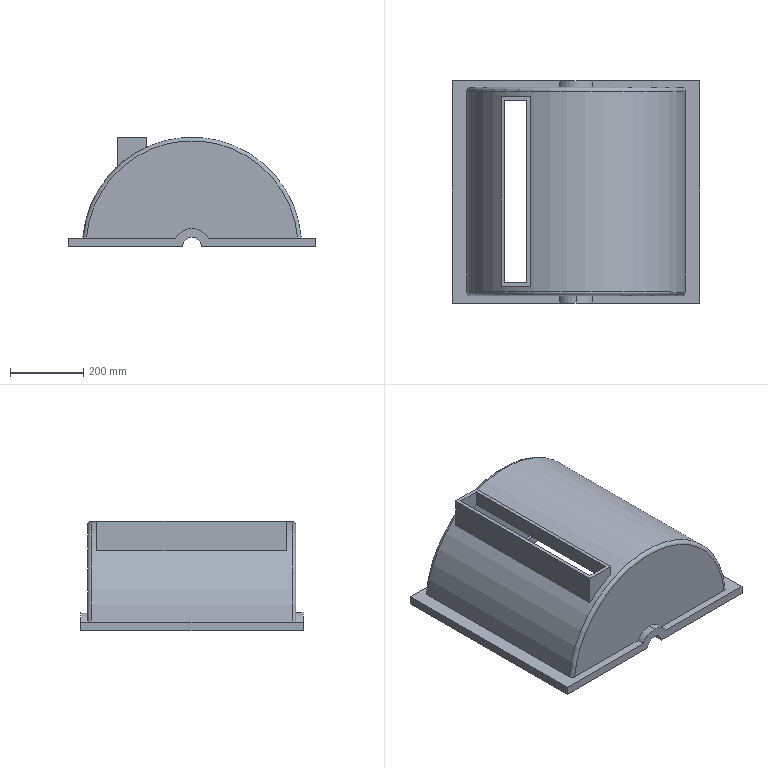Part | SolidWorks | features ICE 11, MirrorPattern 4, Extrusion 1, Fillet 1 | 1 solid | 41 faces | box 677.491 x 608 x 300 mm | volume 10187902 mm3 | plane 25 | cylinder 14 | torus 2 | commonest cylinder face diameters 100 x6 52 x4 556 x2 580 x1 600 x1
STEP:
#1=CARTESIAN_POINT('',(5.246,268.,26.));
#2=VERTEX_POINT('',#1);
#3=CARTESIAN_POINT('',(31.246,268.,0.));
#4=VERTEX_POINT('',#3);
#5=CARTESIAN_POINT('',(5.246,268.,0.));
#6=DIRECTION('',(0.,1.,0.));
#7=DIRECTION('',(0.,0.,1.));
#8=AXIS2_PLACEMENT_3D('',#5,#6,#7);
#9=CIRCLE('',#8,26.);
#10=EDGE_CURVE('',#2,#4,#9,.T.);
#11=ORIENTED_EDGE('',*,*,#10,.F.);
#12=CARTESIAN_POINT('',(5.246,304.,26.));
#13=VERTEX_POINT('',#12);
#14=CARTESIAN_POINT('',(5.246,-304.,26.));
#15=DIRECTION('',(0.,1.,0.));
#16=VECTOR('',#15,1000.);
#17=LINE('',#14,#16);
#18=EDGE_CURVE('',#2,#13,#17,.T.);
#19=ORIENTED_EDGE('',*,*,#18,.T.);
#20=CARTESIAN_POINT('',(31.246,304.,0.));
#21=VERTEX_POINT('',#20);
#22=CARTESIAN_POINT('',(5.246,304.,0.));
#23=DIRECTION('',(0.,1.,0.));
#24=DIRECTION('',(0.,0.,1.));
#25=AXIS2_PLACEMENT_3D('',#22,#23,#24);
#26=CIRCLE('',#25,26.);
#27=EDGE_CURVE('',#13,#21,#26,.T.);
#28=ORIENTED_EDGE('',*,*,#27,.T.);
#29=CARTESIAN_POINT('',(31.246,-304.,0.));
#30=DIRECTION('',(0.,1.,0.));
#31=VECTOR('',#30,1000.);
#32=LINE('',#29,#31);
#33=EDGE_CURVE('',#4,#21,#32,.T.);
#34=ORIENTED_EDGE('',*,*,#33,.F.);
#35=EDGE_LOOP('',(#11,#19,#28,#34));
#36=FACE_OUTER_BOUND('',#35,.T.);
#37=CARTESIAN_POINT('',(5.246,-304.,0.));
#38=DIRECTION('',(0.,1.,0.));
#39=DIRECTION('',(0.,0.,1.));
#40=AXIS2_PLACEMENT_3D('',#37,#38,#39);
#41=CYLINDRICAL_SURFACE('',#40,26.);
#42=ADVANCED_FACE('',(#36),#41,.F.);
#43=CARTESIAN_POINT('',(31.246,-304.,0.));
#44=VERTEX_POINT('',#43);
#45=CARTESIAN_POINT('',(5.246,-304.,26.));
#46=VERTEX_POINT('',#45);
#47=CARTESIAN_POINT('',(5.246,-304.,0.));
#48=DIRECTION('',(0.,-1.,0.));
#49=DIRECTION('',(0.,0.,-1.));
#50=AXIS2_PLACEMENT_3D('',#47,#48,#49);
#51=CIRCLE('',#50,26.);
#52=EDGE_CURVE('',#44,#46,#51,.T.);
#53=ORIENTED_EDGE('',*,*,#52,.T.);
#54=CARTESIAN_POINT('',(5.246,-268.,26.));
#55=VERTEX_POINT('',#54);
#56=CARTESIAN_POINT('',(5.246,-304.,26.));
#57=DIRECTION('',(0.,1.,0.));
#58=VECTOR('',#57,1000.);
#59=LINE('',#56,#58);
#60=EDGE_CURVE('',#46,#55,#59,.T.);
#61=ORIENTED_EDGE('',*,*,#60,.T.);
#62=CARTESIAN_POINT('',(31.246,-268.,0.));
#63=VERTEX_POINT('',#62);
#64=CARTESIAN_POINT('',(5.246,-268.,0.));
#65=DIRECTION('',(0.,-1.,0.));
#66=DIRECTION('',(0.,0.,-1.));
#67=AXIS2_PLACEMENT_3D('',#64,#65,#66);
#68=CIRCLE('',#67,26.);
#69=EDGE_CURVE('',#63,#55,#68,.T.);
#70=ORIENTED_EDGE('',*,*,#69,.F.);
#71=CARTESIAN_POINT('',(31.246,-304.,0.));
#72=DIRECTION('',(0.,1.,0.));
#73=VECTOR('',#72,1000.);
#74=LINE('',#71,#73);
#75=EDGE_CURVE('',#44,#63,#74,.T.);
#76=ORIENTED_EDGE('',*,*,#75,.F.);
#77=EDGE_LOOP('',(#53,#61,#70,#76));
#78=FACE_OUTER_BOUND('',#77,.T.);
#79=CARTESIAN_POINT('',(5.246,-304.,0.));
#80=DIRECTION('',(0.,1.,0.));
#81=DIRECTION('',(0.,0.,1.));
#82=AXIS2_PLACEMENT_3D('',#79,#80,#81);
#83=CYLINDRICAL_SURFACE('',#82,26.);
#84=ADVANCED_FACE('',(#78),#83,.F.);
#85=CARTESIAN_POINT('',(-38.618,-304.,24.));
#86=VERTEX_POINT('',#85);
#87=CARTESIAN_POINT('',(5.246,-304.,50.));
#88=VERTEX_POINT('',#87);
#89=CARTESIAN_POINT('',(5.246,-304.,0.));
#90=DIRECTION('',(0.,1.,0.));
#91=DIRECTION('',(0.,0.,1.));
#92=AXIS2_PLACEMENT_3D('',#89,#90,#91);
#93=CIRCLE('',#92,50.);
#94=EDGE_CURVE('',#86,#88,#93,.T.);
#95=ORIENTED_EDGE('',*,*,#94,.T.);
#96=CARTESIAN_POINT('',(5.246,-284.,50.));
#97=VERTEX_POINT('',#96);
#98=CARTESIAN_POINT('',(5.246,-304.,50.));
#99=DIRECTION('',(0.,1.,0.));
#100=VECTOR('',#99,1000.);
#101=LINE('',#98,#100);
#102=EDGE_CURVE('',#88,#97,#101,.T.);
#103=ORIENTED_EDGE('',*,*,#102,.T.);
#104=CARTESIAN_POINT('',(-38.618,-284.,24.));
#105=VERTEX_POINT('',#104);
#106=CARTESIAN_POINT('',(5.246,-284.,0.));
#107=DIRECTION('',(0.,1.,0.));
#108=DIRECTION('',(0.,0.,-1.));
#109=AXIS2_PLACEMENT_3D('',#106,#107,#108);
#110=CIRCLE('',#109,50.);
#111=EDGE_CURVE('',#105,#97,#110,.T.);
#112=ORIENTED_EDGE('',*,*,#111,.F.);
#113=CARTESIAN_POINT('',(-38.618,-304.,24.));
#114=DIRECTION('',(0.,1.,0.));
#115=VECTOR('',#114,1000.);
#116=LINE('',#113,#115);
#117=EDGE_CURVE('',#86,#105,#116,.T.);
#118=ORIENTED_EDGE('',*,*,#117,.F.);
#119=EDGE_LOOP('',(#95,#103,#112,#118));
#120=FACE_OUTER_BOUND('',#119,.T.);
#121=CARTESIAN_POINT('',(5.246,-304.,0.));
#122=DIRECTION('',(0.,1.,0.));
#123=DIRECTION('',(0.,0.,1.));
#124=AXIS2_PLACEMENT_3D('',#121,#122,#123);
#125=CYLINDRICAL_SURFACE('',#124,50.);
#126=ADVANCED_FACE('',(#120),#125,.T.);
#127=CARTESIAN_POINT('',(-38.618,-274.,24.));
#128=VERTEX_POINT('',#127);
#129=CARTESIAN_POINT('',(5.246,-274.,50.));
#130=VERTEX_POINT('',#129);
#131=CARTESIAN_POINT('',(5.246,-274.,0.));
#132=DIRECTION('',(0.,1.,0.));
#133=DIRECTION('',(0.,0.,-1.));
#134=AXIS2_PLACEMENT_3D('',#131,#132,#133);
#135=CIRCLE('',#134,50.);
#136=EDGE_CURVE('',#128,#130,#135,.T.);
#137=ORIENTED_EDGE('',*,*,#136,.T.);
#138=CARTESIAN_POINT('',(5.246,-268.,50.));
#139=VERTEX_POINT('',#138);
#140=CARTESIAN_POINT('',(5.246,-304.,50.));
#141=DIRECTION('',(0.,1.,0.));
#142=VECTOR('',#141,1000.);
#143=LINE('',#140,#142);
#144=EDGE_CURVE('',#130,#139,#143,.T.);
#145=ORIENTED_EDGE('',*,*,#144,.T.);
#146=CARTESIAN_POINT('',(-38.618,-268.,24.));
#147=VERTEX_POINT('',#146);
#148=CARTESIAN_POINT('',(5.246,-268.,0.));
#149=DIRECTION('',(0.,1.,0.));
#150=DIRECTION('',(0.,0.,-1.));
#151=AXIS2_PLACEMENT_3D('',#148,#149,#150);
#152=CIRCLE('',#151,50.);
#153=EDGE_CURVE('',#147,#139,#152,.T.);
#154=ORIENTED_EDGE('',*,*,#153,.F.);
#155=CARTESIAN_POINT('',(-38.618,-304.,24.));
#156=DIRECTION('',(0.,1.,0.));
#157=VECTOR('',#156,1000.);
#158=LINE('',#155,#157);
#159=EDGE_CURVE('',#128,#147,#158,.T.);
#160=ORIENTED_EDGE('',*,*,#159,.F.);
#161=EDGE_LOOP('',(#137,#145,#154,#160));
#162=FACE_OUTER_BOUND('',#161,.T.);
#163=CARTESIAN_POINT('',(5.246,-304.,0.));
#164=DIRECTION('',(0.,1.,0.));
#165=DIRECTION('',(0.,0.,1.));
#166=AXIS2_PLACEMENT_3D('',#163,#164,#165);
#167=CYLINDRICAL_SURFACE('',#166,50.);
#168=ADVANCED_FACE('',(#162),#167,.T.);
#169=CARTESIAN_POINT('',(-38.618,276.,24.));
#170=VERTEX_POINT('',#169);
#171=CARTESIAN_POINT('',(-283.759,276.,24.));
#172=VERTEX_POINT('',#171);
#173=CARTESIAN_POINT('',(-293.793,276.,24.));
#174=DIRECTION('',(-1.,0.,0.));
#175=VECTOR('',#174,1000.);
#176=LINE('',#173,#175);
#177=EDGE_CURVE('',#170,#172,#176,.T.);
#178=ORIENTED_EDGE('',*,*,#177,.T.);
#179=CARTESIAN_POINT('',(-283.759,-274.,24.));
#180=VERTEX_POINT('',#179);
#181=CARTESIAN_POINT('',(-283.759,286.,24.));
#182=DIRECTION('',(0.,-1.,0.));
#183=VECTOR('',#182,1000.);
#184=LINE('',#181,#183);
#185=EDGE_CURVE('',#172,#180,#184,.T.);
#186=ORIENTED_EDGE('',*,*,#185,.T.);
#187=CARTESIAN_POINT('',(-38.618,-274.,24.));
#188=DIRECTION('',(1.,0.,0.));
#189=VECTOR('',#188,1000.);
#190=LINE('',#187,#189);
#191=EDGE_CURVE('',#180,#128,#190,.T.);
#192=ORIENTED_EDGE('',*,*,#191,.T.);
#193=ORIENTED_EDGE('',*,*,#159,.T.);
#194=CARTESIAN_POINT('',(-276.962,-268.,24.));
#195=VERTEX_POINT('',#194);
#196=CARTESIAN_POINT('',(0.,-268.,24.));
#197=DIRECTION('',(1.,0.,0.));
#198=VECTOR('',#197,1000.);
#199=LINE('',#196,#198);
#200=EDGE_CURVE('',#195,#147,#199,.T.);
#201=ORIENTED_EDGE('',*,*,#200,.F.);
#202=CARTESIAN_POINT('',(-276.962,268.,24.));
#203=VERTEX_POINT('',#202);
#204=CARTESIAN_POINT('',(-276.962,278.,24.));
#205=DIRECTION('',(0.,1.,0.));
#206=VECTOR('',#205,1000.);
#207=LINE('',#204,#206);
#208=EDGE_CURVE('',#195,#203,#207,.T.);
#209=ORIENTED_EDGE('',*,*,#208,.T.);
#210=CARTESIAN_POINT('',(-38.618,268.,24.));
#211=VERTEX_POINT('',#210);
#212=CARTESIAN_POINT('',(0.,268.,24.));
#213=DIRECTION('',(-1.,0.,0.));
#214=VECTOR('',#213,1000.);
#215=LINE('',#212,#214);
#216=EDGE_CURVE('',#211,#203,#215,.T.);
#217=ORIENTED_EDGE('',*,*,#216,.F.);
#218=CARTESIAN_POINT('',(-38.618,304.,24.));
#219=DIRECTION('',(0.,-1.,0.));
#220=VECTOR('',#219,1000.);
#221=LINE('',#218,#220);
#222=EDGE_CURVE('',#170,#211,#221,.T.);
#223=ORIENTED_EDGE('',*,*,#222,.F.);
#224=EDGE_LOOP('',(#178,#186,#192,#193,#201,#209,#217,#223));
#225=FACE_OUTER_BOUND('',#224,.T.);
#226=CARTESIAN_POINT('',(0.,278.,24.));
#227=DIRECTION('',(0.,0.,-1.));
#228=DIRECTION('',(-1.,0.,0.));
#229=AXIS2_PLACEMENT_3D('',#226,#227,#228);
#230=PLANE('',#229);
#231=ADVANCED_FACE('',(#225),#230,.F.);
#232=CARTESIAN_POINT('',(294.251,276.,24.));
#233=VERTEX_POINT('',#232);
#234=CARTESIAN_POINT('',(294.251,-274.,24.));
#235=VERTEX_POINT('',#234);
#236=CARTESIAN_POINT('',(294.251,286.,24.));
#237=DIRECTION('',(0.,-1.,0.));
#238=VECTOR('',#237,1000.);
#239=LINE('',#236,#238);
#240=EDGE_CURVE('',#233,#235,#239,.T.);
#241=ORIENTED_EDGE('',*,*,#240,.F.);
#242=CARTESIAN_POINT('',(49.109,276.,24.));
#243=VERTEX_POINT('',#242);
#244=CARTESIAN_POINT('',(304.284,276.,24.));
#245=DIRECTION('',(-1.,0.,0.));
#246=VECTOR('',#245,1000.);
#247=LINE('',#244,#246);
#248=EDGE_CURVE('',#233,#243,#247,.T.);
#249=ORIENTED_EDGE('',*,*,#248,.T.);
#250=CARTESIAN_POINT('',(49.109,268.,24.));
#251=VERTEX_POINT('',#250);
#252=CARTESIAN_POINT('',(49.109,304.,24.));
#253=DIRECTION('',(0.,-1.,0.));
#254=VECTOR('',#253,1000.);
#255=LINE('',#252,#254);
#256=EDGE_CURVE('',#243,#251,#255,.T.);
#257=ORIENTED_EDGE('',*,*,#256,.T.);
#258=CARTESIAN_POINT('',(287.453,268.,24.));
#259=VERTEX_POINT('',#258);
#260=CARTESIAN_POINT('',(0.,268.,24.));
#261=DIRECTION('',(-1.,0.,0.));
#262=VECTOR('',#261,1000.);
#263=LINE('',#260,#262);
#264=EDGE_CURVE('',#259,#251,#263,.T.);
#265=ORIENTED_EDGE('',*,*,#264,.F.);
#266=CARTESIAN_POINT('',(287.453,-268.,24.));
#267=VERTEX_POINT('',#266);
#268=CARTESIAN_POINT('',(287.453,278.,24.));
#269=DIRECTION('',(0.,1.,0.));
#270=VECTOR('',#269,1000.);
#271=LINE('',#268,#270);
#272=EDGE_CURVE('',#267,#259,#271,.T.);
#273=ORIENTED_EDGE('',*,*,#272,.F.);
#274=CARTESIAN_POINT('',(49.109,-268.,24.));
#275=VERTEX_POINT('',#274);
#276=CARTESIAN_POINT('',(0.,-268.,24.));
#277=DIRECTION('',(1.,0.,0.));
#278=VECTOR('',#277,1000.);
#279=LINE('',#276,#278);
#280=EDGE_CURVE('',#275,#267,#279,.T.);
#281=ORIENTED_EDGE('',*,*,#280,.F.);
#282=CARTESIAN_POINT('',(49.109,-274.,24.));
#283=VERTEX_POINT('',#282);
#284=CARTESIAN_POINT('',(49.109,-304.,24.));
#285=DIRECTION('',(0.,1.,0.));
#286=VECTOR('',#285,1000.);
#287=LINE('',#284,#286);
#288=EDGE_CURVE('',#283,#275,#287,.T.);
#289=ORIENTED_EDGE('',*,*,#288,.F.);
#290=CARTESIAN_POINT('',(49.109,-274.,24.));
#291=DIRECTION('',(1.,0.,0.));
#292=VECTOR('',#291,1000.);
#293=LINE('',#290,#292);
#294=EDGE_CURVE('',#283,#235,#293,.T.);
#295=ORIENTED_EDGE('',*,*,#294,.T.);
#296=EDGE_LOOP('',(#241,#249,#257,#265,#273,#281,#289,#295));
#297=FACE_OUTER_BOUND('',#296,.T.);
#298=CARTESIAN_POINT('',(10.491,278.,24.));
#299=DIRECTION('',(0.,0.,1.));
#300=DIRECTION('',(1.,0.,0.));
#301=AXIS2_PLACEMENT_3D('',#298,#299,#300);
#302=PLANE('',#301);
#303=ADVANCED_FACE('',(#297),#302,.T.);
#304=CARTESIAN_POINT('',(-190.,-249.,214.427));
#305=VERTEX_POINT('',#304);
#306=CARTESIAN_POINT('',(-190.,251.,214.427));
#307=VERTEX_POINT('',#306);
#308=CARTESIAN_POINT('',(-190.,286.,214.427));
#309=DIRECTION('',(0.,1.,0.));
#310=VECTOR('',#309,1000.);
#311=LINE('',#308,#310);
#312=EDGE_CURVE('',#305,#307,#311,.T.);
#313=ORIENTED_EDGE('',*,*,#312,.F.);
#314=CARTESIAN_POINT('',(-129.462,-249.,256.815));
#315=VERTEX_POINT('',#314);
#316=CARTESIAN_POINT('',(5.246,-249.,0.));
#317=DIRECTION('',(0.,-1.,0.));
#318=DIRECTION('',(0.,0.,-1.));
#319=AXIS2_PLACEMENT_3D('',#316,#317,#318);
#320=CIRCLE('',#319,290.);
#321=EDGE_CURVE('',#315,#305,#320,.T.);
#322=ORIENTED_EDGE('',*,*,#321,.F.);
#323=CARTESIAN_POINT('',(-129.462,251.,256.815));
#324=VERTEX_POINT('',#323);
#325=CARTESIAN_POINT('',(-129.462,286.,256.815));
#326=DIRECTION('',(0.,-1.,0.));
#327=VECTOR('',#326,1000.);
#328=LINE('',#325,#327);
#329=EDGE_CURVE('',#324,#315,#328,.T.);
#330=ORIENTED_EDGE('',*,*,#329,.F.);
#331=CARTESIAN_POINT('',(5.246,251.,0.));
#332=DIRECTION('',(0.,1.,0.));
#333=DIRECTION('',(0.,0.,1.));
#334=AXIS2_PLACEMENT_3D('',#331,#332,#333);
#335=CIRCLE('',#334,290.);
#336=EDGE_CURVE('',#307,#324,#335,.T.);
#337=ORIENTED_EDGE('',*,*,#336,.F.);
#338=EDGE_LOOP('',(#313,#322,#330,#337));
#339=FACE_BOUND('',#338,.T.);
#340=ORIENTED_EDGE('',*,*,#185,.F.);
#341=CARTESIAN_POINT('',(5.246,276.,0.));
#342=DIRECTION('',(0.,1.,0.));
#343=DIRECTION('',(0.,0.,1.));
#344=AXIS2_PLACEMENT_3D('',#341,#342,#343);
#345=CIRCLE('',#344,290.);
#346=EDGE_CURVE('',#172,#233,#345,.T.);
#347=ORIENTED_EDGE('',*,*,#346,.T.);
#348=ORIENTED_EDGE('',*,*,#240,.T.);
#349=CARTESIAN_POINT('',(5.246,-274.,0.));
#350=DIRECTION('',(0.,-1.,0.));
#351=DIRECTION('',(0.,0.,-1.));
#352=AXIS2_PLACEMENT_3D('',#349,#350,#351);
#353=CIRCLE('',#352,290.);
#354=EDGE_CURVE('',#235,#180,#353,.T.);
#355=ORIENTED_EDGE('',*,*,#354,.T.);
#356=EDGE_LOOP('',(#340,#347,#348,#355));
#357=FACE_OUTER_BOUND('',#356,.T.);
#358=CARTESIAN_POINT('',(5.246,286.,0.));
#359=DIRECTION('',(0.,-1.,0.));
#360=DIRECTION('',(0.,0.,-1.));
#361=AXIS2_PLACEMENT_3D('',#358,#359,#360);
#362=CYLINDRICAL_SURFACE('',#361,290.);
#363=ADVANCED_FACE('',(#339,#357),#362,.F.);
#364=CARTESIAN_POINT('',(5.246,276.,0.));
#365=DIRECTION('',(0.,-1.,0.));
#366=DIRECTION('',(0.,0.,1.));
#367=AXIS2_PLACEMENT_3D('',#364,#365,#366);
#368=CIRCLE('',#367,50.);
#369=EDGE_CURVE('',#243,#170,#368,.T.);
#370=ORIENTED_EDGE('',*,*,#369,.T.);
#371=ORIENTED_EDGE('',*,*,#222,.T.);
#372=CARTESIAN_POINT('',(5.246,268.,0.));
#373=DIRECTION('',(0.,-1.,0.));
#374=DIRECTION('',(0.,0.,1.));
#375=AXIS2_PLACEMENT_3D('',#372,#373,#374);
#376=CIRCLE('',#375,50.);
#377=EDGE_CURVE('',#251,#211,#376,.T.);
#378=ORIENTED_EDGE('',*,*,#377,.F.);
#379=ORIENTED_EDGE('',*,*,#256,.F.);
#380=EDGE_LOOP('',(#370,#371,#378,#379));
#381=FACE_OUTER_BOUND('',#380,.T.);
#382=CARTESIAN_POINT('',(5.246,304.,0.));
#383=DIRECTION('',(0.,-1.,0.));
#384=DIRECTION('',(0.,0.,-1.));
#385=AXIS2_PLACEMENT_3D('',#382,#383,#384);
#386=CYLINDRICAL_SURFACE('',#385,50.);
#387=ADVANCED_FACE('',(#381),#386,.T.);
#388=CARTESIAN_POINT('',(-38.618,286.,24.));
#389=VERTEX_POINT('',#388);
#390=CARTESIAN_POINT('',(-283.759,286.,24.));
#391=VERTEX_POINT('',#390);
#392=CARTESIAN_POINT('',(0.,286.,24.));
#393=DIRECTION('',(-1.,0.,0.));
#394=VECTOR('',#393,1000.);
#395=LINE('',#392,#394);
#396=EDGE_CURVE('',#389,#391,#395,.T.);
#397=ORIENTED_EDGE('',*,*,#396,.F.);
#398=CARTESIAN_POINT('',(-38.618,304.,24.));
#399=VERTEX_POINT('',#398);
#400=CARTESIAN_POINT('',(-38.618,304.,24.));
#401=DIRECTION('',(0.,-1.,0.));
#402=VECTOR('',#401,1000.);
#403=LINE('',#400,#402);
#404=EDGE_CURVE('',#399,#389,#403,.T.);
#405=ORIENTED_EDGE('',*,*,#404,.F.);
#406=CARTESIAN_POINT('',(-333.5,304.,24.));
#407=VERTEX_POINT('',#406);
#408=CARTESIAN_POINT('',(-333.5,304.,24.));
#409=DIRECTION('',(1.,0.,0.));
#410=VECTOR('',#409,1000.);
#411=LINE('',#408,#410);
#412=EDGE_CURVE('',#407,#399,#411,.T.);
#413=ORIENTED_EDGE('',*,*,#412,.F.);
#414=CARTESIAN_POINT('',(-333.5,-304.,24.));
#415=VERTEX_POINT('',#414);
#416=CARTESIAN_POINT('',(-333.5,278.,24.));
#417=DIRECTION('',(0.,-1.,0.));
#418=VECTOR('',#417,1000.);
#419=LINE('',#416,#418);
#420=EDGE_CURVE('',#407,#415,#419,.T.);
#421=ORIENTED_EDGE('',*,*,#420,.T.);
#422=CARTESIAN_POINT('',(-333.5,-304.,24.));
#423=DIRECTION('',(1.,0.,0.));
#424=VECTOR('',#423,1000.);
#425=LINE('',#422,#424);
#426=EDGE_CURVE('',#415,#86,#425,.T.);
#427=ORIENTED_EDGE('',*,*,#426,.T.);
#428=ORIENTED_EDGE('',*,*,#117,.T.);
#429=CARTESIAN_POINT('',(-283.759,-284.,24.));
#430=VERTEX_POINT('',#429);
#431=CARTESIAN_POINT('',(0.,-284.,24.));
#432=DIRECTION('',(-1.,0.,0.));
#433=VECTOR('',#432,1000.);
#434=LINE('',#431,#433);
#435=EDGE_CURVE('',#105,#430,#434,.T.);
#436=ORIENTED_EDGE('',*,*,#435,.T.);
#437=CARTESIAN_POINT('',(-293.793,-274.,24.));
#438=VERTEX_POINT('',#437);
#439=CARTESIAN_POINT('',(-283.759,-284.,24.));
#440=CARTESIAN_POINT('',(-284.421,-284.,24.));
#441=CARTESIAN_POINT('',(-285.071,-283.935,24.));
#442=CARTESIAN_POINT('',(-286.031,-283.746,24.));
#443=CARTESIAN_POINT('',(-286.348,-283.667,24.));
#444=CARTESIAN_POINT('',(-286.977,-283.477,24.));
#445=CARTESIAN_POINT('',(-287.29,-283.366,24.));
#446=CARTESIAN_POINT('',(-288.2,-282.991,24.));
#447=CARTESIAN_POINT('',(-288.776,-282.685,24.));
#448=CARTESIAN_POINT('',(-289.866,-281.962,24.));
#449=CARTESIAN_POINT('',(-290.383,-281.54,24.));
#450=CARTESIAN_POINT('',(-291.309,-280.619,24.));
#451=CARTESIAN_POINT('',(-291.725,-280.116,24.));
#452=CARTESIAN_POINT('',(-292.276,-279.298,24.));
#453=CARTESIAN_POINT('',(-292.447,-279.014,24.));
#454=CARTESIAN_POINT('',(-292.758,-278.436,24.));
#455=CARTESIAN_POINT('',(-293.038,-277.847,24.));
#456=CARTESIAN_POINT('',(-293.26,-277.233,24.));
#457=CARTESIAN_POINT('',(-293.451,-276.607,24.));
#458=CARTESIAN_POINT('',(-293.533,-276.286,24.));
#459=CARTESIAN_POINT('',(-293.728,-275.316,24.));
#460=CARTESIAN_POINT('',(-293.793,-274.661,24.));
#461=CARTESIAN_POINT('',(-293.793,-274.,24.));
#462=B_SPLINE_CURVE_WITH_KNOTS('',3,(#439,#440,#441,#442,#443,#444,#445,#446,#447,#448,#449,#450,#451,#452,#453,#454,#455,#456,#457,#458,#459,#460,#461),.UNSPECIFIED.,.F.,.F.,(4,2,2,2,2,2,2,2,1,2,2,4),(0.,0.001956,0.002934,0.003912,0.005868,0.007824,0.00978,0.01076,0.01174,0.01271,0.01369,0.01565),.UNSPECIFIED.);
#463=EDGE_CURVE('',#430,#438,#462,.T.);
#464=ORIENTED_EDGE('',*,*,#463,.T.);
#465=CARTESIAN_POINT('',(-293.793,276.,24.));
#466=VERTEX_POINT('',#465);
#467=CARTESIAN_POINT('',(-293.793,286.,24.));
#468=DIRECTION('',(0.,1.,0.));
#469=VECTOR('',#468,1000.);
#470=LINE('',#467,#469);
#471=EDGE_CURVE('',#438,#466,#470,.T.);
#472=ORIENTED_EDGE('',*,*,#471,.T.);
#473=CARTESIAN_POINT('',(-293.793,276.,24.));
#474=CARTESIAN_POINT('',(-293.793,276.661,24.));
#475=CARTESIAN_POINT('',(-293.728,277.312,24.));
#476=CARTESIAN_POINT('',(-293.536,278.271,24.));
#477=CARTESIAN_POINT('',(-293.457,278.588,24.));
#478=CARTESIAN_POINT('',(-293.265,279.217,24.));
#479=CARTESIAN_POINT('',(-293.153,279.529,24.));
#480=CARTESIAN_POINT('',(-292.775,280.438,24.));
#481=CARTESIAN_POINT('',(-292.466,281.012,24.));
#482=CARTESIAN_POINT('',(-291.92,281.828,24.));
#483=CARTESIAN_POINT('',(-291.723,282.093,24.));
#484=CARTESIAN_POINT('',(-291.303,282.602,24.));
#485=CARTESIAN_POINT('',(-291.082,282.844,24.));
#486=CARTESIAN_POINT('',(-290.388,283.535,24.));
#487=CARTESIAN_POINT('',(-289.883,283.949,24.));
#488=CARTESIAN_POINT('',(-289.061,284.496,24.));
#489=CARTESIAN_POINT('',(-288.777,284.666,24.));
#490=CARTESIAN_POINT('',(-288.198,284.974,24.));
#491=CARTESIAN_POINT('',(-287.608,285.252,24.));
#492=CARTESIAN_POINT('',(-286.993,285.472,24.));
#493=CARTESIAN_POINT('',(-286.366,285.662,24.));
#494=CARTESIAN_POINT('',(-286.045,285.743,24.));
#495=CARTESIAN_POINT('',(-285.075,285.935,24.));
#496=CARTESIAN_POINT('',(-284.421,286.,24.));
#497=CARTESIAN_POINT('',(-283.759,286.,24.));
#498=B_SPLINE_CURVE_WITH_KNOTS('',3,(#473,#474,#475,#476,#477,#478,#479,#480,#481,#482,#483,#484,#485,#486,#487,#488,#489,#490,#491,#492,#493,#494,#495,#496,#497),.UNSPECIFIED.,.F.,.F.,(4,2,2,2,2,2,2,2,2,1,2,2,4),(0.,0.001956,0.002934,0.003912,0.005868,0.006846,0.007824,0.00978,0.01076,0.01174,0.01271,0.01369,0.01565),.UNSPECIFIED.);
#499=EDGE_CURVE('',#466,#391,#498,.T.);
#500=ORIENTED_EDGE('',*,*,#499,.T.);
#501=EDGE_LOOP('',(#397,#405,#413,#421,#427,#428,#436,#464,#472,#500));
#502=FACE_OUTER_BOUND('',#501,.T.);
#503=CARTESIAN_POINT('',(0.,278.,24.));
#504=DIRECTION('',(0.,0.,-1.));
#505=DIRECTION('',(-1.,0.,0.));
#506=AXIS2_PLACEMENT_3D('',#503,#504,#505);
#507=PLANE('',#506);
#508=ADVANCED_FACE('',(#502),#507,.F.);
#509=CARTESIAN_POINT('',(49.109,304.,24.));
#510=VERTEX_POINT('',#509);
#511=CARTESIAN_POINT('',(49.109,286.,24.));
#512=VERTEX_POINT('',#511);
#513=CARTESIAN_POINT('',(49.109,304.,24.));
#514=DIRECTION('',(0.,-1.,0.));
#515=VECTOR('',#514,1000.);
#516=LINE('',#513,#515);
#517=EDGE_CURVE('',#510,#512,#516,.T.);
#518=ORIENTED_EDGE('',*,*,#517,.T.);
#519=CARTESIAN_POINT('',(294.251,286.,24.));
#520=VERTEX_POINT('',#519);
#521=CARTESIAN_POINT('',(10.491,286.,24.));
#522=DIRECTION('',(1.,0.,0.));
#523=VECTOR('',#522,1000.);
#524=LINE('',#521,#523);
#525=EDGE_CURVE('',#512,#520,#524,.T.);
#526=ORIENTED_EDGE('',*,*,#525,.T.);
#527=CARTESIAN_POINT('',(304.284,276.,24.));
#528=VERTEX_POINT('',#527);
#529=CARTESIAN_POINT('',(294.251,286.,24.));
#530=CARTESIAN_POINT('',(294.912,286.,24.));
#531=CARTESIAN_POINT('',(295.563,285.935,24.));
#532=CARTESIAN_POINT('',(296.522,285.746,24.));
#533=CARTESIAN_POINT('',(296.84,285.667,24.));
#534=CARTESIAN_POINT('',(297.469,285.477,24.));
#535=CARTESIAN_POINT('',(297.782,285.366,24.));
#536=CARTESIAN_POINT('',(298.692,284.991,24.));
#537=CARTESIAN_POINT('',(299.268,284.685,24.));
#538=CARTESIAN_POINT('',(300.357,283.962,24.));
#539=CARTESIAN_POINT('',(300.874,283.54,24.));
#540=CARTESIAN_POINT('',(301.8,282.619,24.));
#541=CARTESIAN_POINT('',(302.216,282.116,24.));
#542=CARTESIAN_POINT('',(302.767,281.298,24.));
#543=CARTESIAN_POINT('',(302.938,281.014,24.));
#544=CARTESIAN_POINT('',(303.249,280.436,24.));
#545=CARTESIAN_POINT('',(303.53,279.847,24.));
#546=CARTESIAN_POINT('',(303.751,279.233,24.));
#547=CARTESIAN_POINT('',(303.943,278.607,24.));
#548=CARTESIAN_POINT('',(304.024,278.286,24.));
#549=CARTESIAN_POINT('',(304.219,277.316,24.));
#550=CARTESIAN_POINT('',(304.284,276.661,24.));
#551=CARTESIAN_POINT('',(304.284,276.,24.));
#552=B_SPLINE_CURVE_WITH_KNOTS('',3,(#529,#530,#531,#532,#533,#534,#535,#536,#537,#538,#539,#540,#541,#542,#543,#544,#545,#546,#547,#548,#549,#550,#551),.UNSPECIFIED.,.F.,.F.,(4,2,2,2,2,2,2,2,1,2,2,4),(0.,0.001956,0.002934,0.003912,0.005868,0.007824,0.00978,0.01076,0.01174,0.01271,0.01369,0.01565),.UNSPECIFIED.);
#553=EDGE_CURVE('',#520,#528,#552,.T.);
#554=ORIENTED_EDGE('',*,*,#553,.T.);
#555=CARTESIAN_POINT('',(304.284,-274.,24.));
#556=VERTEX_POINT('',#555);
#557=CARTESIAN_POINT('',(304.284,286.,24.));
#558=DIRECTION('',(0.,1.,0.));
#559=VECTOR('',#558,1000.);
#560=LINE('',#557,#559);
#561=EDGE_CURVE('',#556,#528,#560,.T.);
#562=ORIENTED_EDGE('',*,*,#561,.F.);
#563=CARTESIAN_POINT('',(294.251,-284.,24.));
#564=VERTEX_POINT('',#563);
#565=CARTESIAN_POINT('',(304.284,-274.,24.));
#566=CARTESIAN_POINT('',(304.284,-274.661,24.));
#567=CARTESIAN_POINT('',(304.219,-275.312,24.));
#568=CARTESIAN_POINT('',(304.027,-276.271,24.));
#569=CARTESIAN_POINT('',(303.948,-276.588,24.));
#570=CARTESIAN_POINT('',(303.757,-277.217,24.));
#571=CARTESIAN_POINT('',(303.644,-277.529,24.));
#572=CARTESIAN_POINT('',(303.266,-278.438,24.));
#573=CARTESIAN_POINT('',(302.958,-279.012,24.));
#574=CARTESIAN_POINT('',(302.411,-279.828,24.));
#575=CARTESIAN_POINT('',(302.214,-280.093,24.));
#576=CARTESIAN_POINT('',(301.794,-280.602,24.));
#577=CARTESIAN_POINT('',(301.574,-280.844,24.));
#578=CARTESIAN_POINT('',(300.88,-281.535,24.));
#579=CARTESIAN_POINT('',(300.375,-281.949,24.));
#580=CARTESIAN_POINT('',(299.553,-282.496,24.));
#581=CARTESIAN_POINT('',(299.268,-282.666,24.));
#582=CARTESIAN_POINT('',(298.69,-282.974,24.));
#583=CARTESIAN_POINT('',(298.099,-283.252,24.));
#584=CARTESIAN_POINT('',(297.485,-283.472,24.));
#585=CARTESIAN_POINT('',(296.858,-283.662,24.));
#586=CARTESIAN_POINT('',(296.537,-283.743,24.));
#587=CARTESIAN_POINT('',(295.566,-283.935,24.));
#588=CARTESIAN_POINT('',(294.912,-284.,24.));
#589=CARTESIAN_POINT('',(294.251,-284.,24.));
#590=B_SPLINE_CURVE_WITH_KNOTS('',3,(#565,#566,#567,#568,#569,#570,#571,#572,#573,#574,#575,#576,#577,#578,#579,#580,#581,#582,#583,#584,#585,#586,#587,#588,#589),.UNSPECIFIED.,.F.,.F.,(4,2,2,2,2,2,2,2,2,1,2,2,4),(0.,0.001956,0.002934,0.003912,0.005868,0.006846,0.007824,0.00978,0.01076,0.01174,0.01271,0.01369,0.01565),.UNSPECIFIED.);
#591=EDGE_CURVE('',#556,#564,#590,.T.);
#592=ORIENTED_EDGE('',*,*,#591,.T.);
#593=CARTESIAN_POINT('',(49.109,-284.,24.));
#594=VERTEX_POINT('',#593);
#595=CARTESIAN_POINT('',(10.491,-284.,24.));
#596=DIRECTION('',(1.,0.,0.));
#597=VECTOR('',#596,1000.);
#598=LINE('',#595,#597);
#599=EDGE_CURVE('',#594,#564,#598,.T.);
#600=ORIENTED_EDGE('',*,*,#599,.F.);
#601=CARTESIAN_POINT('',(49.109,-304.,24.));
#602=VERTEX_POINT('',#601);
#603=CARTESIAN_POINT('',(49.109,-304.,24.));
#604=DIRECTION('',(0.,1.,0.));
#605=VECTOR('',#604,1000.);
#606=LINE('',#603,#605);
#607=EDGE_CURVE('',#602,#594,#606,.T.);
#608=ORIENTED_EDGE('',*,*,#607,.F.);
#609=CARTESIAN_POINT('',(343.991,-304.,24.));
#610=VERTEX_POINT('',#609);
#611=CARTESIAN_POINT('',(343.991,-304.,24.));
#612=DIRECTION('',(-1.,0.,0.));
#613=VECTOR('',#612,1000.);
#614=LINE('',#611,#613);
#615=EDGE_CURVE('',#610,#602,#614,.T.);
#616=ORIENTED_EDGE('',*,*,#615,.F.);
#617=CARTESIAN_POINT('',(343.991,304.,24.));
#618=VERTEX_POINT('',#617);
#619=CARTESIAN_POINT('',(343.991,278.,24.));
#620=DIRECTION('',(0.,-1.,0.));
#621=VECTOR('',#620,1000.);
#622=LINE('',#619,#621);
#623=EDGE_CURVE('',#618,#610,#622,.T.);
#624=ORIENTED_EDGE('',*,*,#623,.F.);
#625=CARTESIAN_POINT('',(343.991,304.,24.));
#626=DIRECTION('',(1.,0.,0.));
#627=VECTOR('',#626,1000.);
#628=LINE('',#625,#627);
#629=EDGE_CURVE('',#510,#618,#628,.T.);
#630=ORIENTED_EDGE('',*,*,#629,.F.);
#631=EDGE_LOOP('',(#518,#526,#554,#562,#592,#600,#608,#616,#624,#630));
#632=FACE_OUTER_BOUND('',#631,.T.);
#633=CARTESIAN_POINT('',(10.491,278.,24.));
#634=DIRECTION('',(0.,0.,1.));
#635=DIRECTION('',(1.,0.,0.));
#636=AXIS2_PLACEMENT_3D('',#633,#634,#635);
#637=PLANE('',#636);
#638=ADVANCED_FACE('',(#632),#637,.T.);
#639=ORIENTED_EDGE('',*,*,#144,.F.);
#640=CARTESIAN_POINT('',(5.246,-274.,0.));
#641=DIRECTION('',(0.,1.,0.));
#642=DIRECTION('',(0.,0.,-1.));
#643=AXIS2_PLACEMENT_3D('',#640,#641,#642);
#644=CIRCLE('',#643,50.);
#645=EDGE_CURVE('',#130,#283,#644,.T.);
#646=ORIENTED_EDGE('',*,*,#645,.T.);
#647=ORIENTED_EDGE('',*,*,#288,.T.);
#648=CARTESIAN_POINT('',(5.246,-268.,0.));
#649=DIRECTION('',(0.,1.,0.));
#650=DIRECTION('',(0.,0.,-1.));
#651=AXIS2_PLACEMENT_3D('',#648,#649,#650);
#652=CIRCLE('',#651,50.);
#653=EDGE_CURVE('',#139,#275,#652,.T.);
#654=ORIENTED_EDGE('',*,*,#653,.F.);
#655=EDGE_LOOP('',(#639,#646,#647,#654));
#656=FACE_OUTER_BOUND('',#655,.T.);
#657=CARTESIAN_POINT('',(5.246,-304.,0.));
#658=DIRECTION('',(0.,1.,0.));
#659=DIRECTION('',(0.,0.,1.));
#660=AXIS2_PLACEMENT_3D('',#657,#658,#659);
#661=CYLINDRICAL_SURFACE('',#660,50.);
#662=ADVANCED_FACE('',(#656),#661,.T.);
#663=CARTESIAN_POINT('',(343.991,-304.,0.));
#664=VERTEX_POINT('',#663);
#665=CARTESIAN_POINT('',(-333.5,-304.,0.));
#666=DIRECTION('',(1.,0.,0.));
#667=VECTOR('',#666,1000.);
#668=LINE('',#665,#667);
#669=EDGE_CURVE('',#44,#664,#668,.T.);
#670=ORIENTED_EDGE('',*,*,#669,.F.);
#671=ORIENTED_EDGE('',*,*,#75,.T.);
#672=CARTESIAN_POINT('',(288.491,-268.,0.));
#673=VERTEX_POINT('',#672);
#674=CARTESIAN_POINT('',(-298.,-268.,0.));
#675=DIRECTION('',(-1.,0.,0.));
#676=VECTOR('',#675,1000.);
#677=LINE('',#674,#676);
#678=EDGE_CURVE('',#673,#63,#677,.T.);
#679=ORIENTED_EDGE('',*,*,#678,.F.);
#680=CARTESIAN_POINT('',(288.491,268.,0.));
#681=VERTEX_POINT('',#680);
#682=CARTESIAN_POINT('',(288.491,278.,0.));
#683=DIRECTION('',(0.,-1.,0.));
#684=VECTOR('',#683,1000.);
#685=LINE('',#682,#684);
#686=EDGE_CURVE('',#681,#673,#685,.T.);
#687=ORIENTED_EDGE('',*,*,#686,.F.);
#688=CARTESIAN_POINT('',(-298.,268.,0.));
#689=DIRECTION('',(-1.,0.,0.));
#690=VECTOR('',#689,1000.);
#691=LINE('',#688,#690);
#692=EDGE_CURVE('',#681,#4,#691,.T.);
#693=ORIENTED_EDGE('',*,*,#692,.T.);
#694=ORIENTED_EDGE('',*,*,#33,.T.);
#695=CARTESIAN_POINT('',(343.991,304.,0.));
#696=VERTEX_POINT('',#695);
#697=CARTESIAN_POINT('',(-333.5,304.,0.));
#698=DIRECTION('',(1.,0.,0.));
#699=VECTOR('',#698,1000.);
#700=LINE('',#697,#699);
#701=EDGE_CURVE('',#21,#696,#700,.T.);
#702=ORIENTED_EDGE('',*,*,#701,.T.);
#703=CARTESIAN_POINT('',(343.991,278.,0.));
#704=DIRECTION('',(0.,-1.,0.));
#705=VECTOR('',#704,1000.);
#706=LINE('',#703,#705);
#707=EDGE_CURVE('',#696,#664,#706,.T.);
#708=ORIENTED_EDGE('',*,*,#707,.T.);
#709=EDGE_LOOP('',(#670,#671,#679,#687,#693,#694,#702,#708));
#710=FACE_OUTER_BOUND('',#709,.T.);
#711=CARTESIAN_POINT('',(0.,278.,0.));
#712=DIRECTION('',(0.,0.,1.));
#713=DIRECTION('',(1.,0.,0.));
#714=AXIS2_PLACEMENT_3D('',#711,#712,#713);
#715=PLANE('',#714);
#716=ADVANCED_FACE('',(#710),#715,.F.);
#717=ORIENTED_EDGE('',*,*,#208,.F.);
#718=CARTESIAN_POINT('',(-278.,-268.,0.));
#719=VERTEX_POINT('',#718);
#720=CARTESIAN_POINT('',(0.,-268.,0.));
#721=DIRECTION('',(0.,-1.,0.));
#722=DIRECTION('',(0.,0.,-1.));
#723=AXIS2_PLACEMENT_3D('',#720,#721,#722);
#724=CIRCLE('',#723,278.);
#725=EDGE_CURVE('',#195,#719,#724,.T.);
#726=ORIENTED_EDGE('',*,*,#725,.T.);
#727=CARTESIAN_POINT('',(-278.,268.,0.));
#728=VERTEX_POINT('',#727);
#729=CARTESIAN_POINT('',(-278.,278.,0.));
#730=DIRECTION('',(0.,-1.,0.));
#731=VECTOR('',#730,1000.);
#732=LINE('',#729,#731);
#733=EDGE_CURVE('',#728,#719,#732,.T.);
#734=ORIENTED_EDGE('',*,*,#733,.F.);
#735=CARTESIAN_POINT('',(0.,268.,0.));
#736=DIRECTION('',(0.,1.,0.));
#737=DIRECTION('',(0.,0.,1.));
#738=AXIS2_PLACEMENT_3D('',#735,#736,#737);
#739=CIRCLE('',#738,278.);
#740=EDGE_CURVE('',#728,#203,#739,.T.);
#741=ORIENTED_EDGE('',*,*,#740,.T.);
#742=EDGE_LOOP('',(#717,#726,#734,#741));
#743=FACE_OUTER_BOUND('',#742,.T.);
#744=CARTESIAN_POINT('',(0.,278.,0.));
#745=DIRECTION('',(0.,-1.,0.));
#746=DIRECTION('',(0.,0.,-1.));
#747=AXIS2_PLACEMENT_3D('',#744,#745,#746);
#748=CYLINDRICAL_SURFACE('',#747,278.);
#749=ADVANCED_FACE('',(#743),#748,.F.);
#750=CARTESIAN_POINT('',(-333.5,304.,0.));
#751=VERTEX_POINT('',#750);
#752=CARTESIAN_POINT('',(-20.754,304.,0.));
#753=VERTEX_POINT('',#752);
#754=CARTESIAN_POINT('',(-333.5,304.,0.));
#755=DIRECTION('',(1.,0.,0.));
#756=VECTOR('',#755,1000.);
#757=LINE('',#754,#756);
#758=EDGE_CURVE('',#751,#753,#757,.T.);
#759=ORIENTED_EDGE('',*,*,#758,.T.);
#760=CARTESIAN_POINT('',(-20.754,268.,0.));
#761=VERTEX_POINT('',#760);
#762=CARTESIAN_POINT('',(-20.754,-304.,0.));
#763=DIRECTION('',(0.,-1.,0.));
#764=VECTOR('',#763,1000.);
#765=LINE('',#762,#764);
#766=EDGE_CURVE('',#753,#761,#765,.T.);
#767=ORIENTED_EDGE('',*,*,#766,.T.);
#768=CARTESIAN_POINT('',(-298.,268.,0.));
#769=DIRECTION('',(-1.,0.,0.));
#770=VECTOR('',#769,1000.);
#771=LINE('',#768,#770);
#772=EDGE_CURVE('',#761,#728,#771,.T.);
#773=ORIENTED_EDGE('',*,*,#772,.T.);
#774=ORIENTED_EDGE('',*,*,#733,.T.);
#775=CARTESIAN_POINT('',(-20.754,-268.,0.));
#776=VERTEX_POINT('',#775);
#777=CARTESIAN_POINT('',(-298.,-268.,0.));
#778=DIRECTION('',(-1.,0.,0.));
#779=VECTOR('',#778,1000.);
#780=LINE('',#777,#779);
#781=EDGE_CURVE('',#776,#719,#780,.T.);
#782=ORIENTED_EDGE('',*,*,#781,.F.);
#783=CARTESIAN_POINT('',(-20.754,-304.,0.));
#784=VERTEX_POINT('',#783);
#785=CARTESIAN_POINT('',(-20.754,-304.,0.));
#786=DIRECTION('',(0.,-1.,0.));
#787=VECTOR('',#786,1000.);
#788=LINE('',#785,#787);
#789=EDGE_CURVE('',#776,#784,#788,.T.);
#790=ORIENTED_EDGE('',*,*,#789,.T.);
#791=CARTESIAN_POINT('',(-333.5,-304.,0.));
#792=VERTEX_POINT('',#791);
#793=CARTESIAN_POINT('',(-333.5,-304.,0.));
#794=DIRECTION('',(1.,0.,0.));
#795=VECTOR('',#794,1000.);
#796=LINE('',#793,#795);
#797=EDGE_CURVE('',#792,#784,#796,.T.);
#798=ORIENTED_EDGE('',*,*,#797,.F.);
#799=CARTESIAN_POINT('',(-333.5,278.,0.));
#800=DIRECTION('',(0.,-1.,0.));
#801=VECTOR('',#800,1000.);
#802=LINE('',#799,#801);
#803=EDGE_CURVE('',#751,#792,#802,.T.);
#804=ORIENTED_EDGE('',*,*,#803,.F.);
#805=EDGE_LOOP('',(#759,#767,#773,#774,#782,#790,#798,#804));
#806=FACE_OUTER_BOUND('',#805,.T.);
#807=CARTESIAN_POINT('',(0.,278.,0.));
#808=DIRECTION('',(0.,0.,1.));
#809=DIRECTION('',(1.,0.,0.));
#810=AXIS2_PLACEMENT_3D('',#807,#808,#809);
#811=PLANE('',#810);
#812=ADVANCED_FACE('',(#806),#811,.F.);
#813=ORIENTED_EDGE('',*,*,#803,.T.);
#814=CARTESIAN_POINT('',(-333.5,-304.,24.));
#815=DIRECTION('',(0.,0.,-1.));
#816=VECTOR('',#815,1000.);
#817=LINE('',#814,#816);
#818=EDGE_CURVE('',#415,#792,#817,.T.);
#819=ORIENTED_EDGE('',*,*,#818,.F.);
#820=ORIENTED_EDGE('',*,*,#420,.F.);
#821=CARTESIAN_POINT('',(-333.5,304.,24.));
#822=DIRECTION('',(0.,0.,-1.));
#823=VECTOR('',#822,1000.);
#824=LINE('',#821,#823);
#825=EDGE_CURVE('',#407,#751,#824,.T.);
#826=ORIENTED_EDGE('',*,*,#825,.T.);
#827=EDGE_LOOP('',(#813,#819,#820,#826));
#828=FACE_OUTER_BOUND('',#827,.T.);
#829=CARTESIAN_POINT('',(-333.5,278.,0.));
#830=DIRECTION('',(1.,0.,0.));
#831=DIRECTION('',(0.,0.,-1.));
#832=AXIS2_PLACEMENT_3D('',#829,#830,#831);
#833=PLANE('',#832);
#834=ADVANCED_FACE('',(#828),#833,.F.);
#835=ORIENTED_EDGE('',*,*,#377,.T.);
#836=ORIENTED_EDGE('',*,*,#216,.T.);
#837=ORIENTED_EDGE('',*,*,#740,.F.);
#838=ORIENTED_EDGE('',*,*,#772,.F.);
#839=CARTESIAN_POINT('',(5.246,268.,0.));
#840=DIRECTION('',(0.,1.,0.));
#841=DIRECTION('',(0.,0.,1.));
#842=AXIS2_PLACEMENT_3D('',#839,#840,#841);
#843=CIRCLE('',#842,26.);
#844=EDGE_CURVE('',#761,#2,#843,.T.);
#845=ORIENTED_EDGE('',*,*,#844,.T.);
#846=ORIENTED_EDGE('',*,*,#10,.T.);
#847=ORIENTED_EDGE('',*,*,#692,.F.);
#848=CARTESIAN_POINT('',(10.491,268.,0.));
#849=DIRECTION('',(0.,1.,0.));
#850=DIRECTION('',(0.,0.,1.));
#851=AXIS2_PLACEMENT_3D('',#848,#849,#850);
#852=CIRCLE('',#851,278.);
#853=EDGE_CURVE('',#259,#681,#852,.T.);
#854=ORIENTED_EDGE('',*,*,#853,.F.);
#855=ORIENTED_EDGE('',*,*,#264,.T.);
#856=EDGE_LOOP('',(#835,#836,#837,#838,#845,#846,#847,#854,#855));
#857=FACE_OUTER_BOUND('',#856,.T.);
#858=CARTESIAN_POINT('',(0.,268.,0.));
#859=DIRECTION('',(0.,1.,0.));
#860=DIRECTION('',(0.,0.,1.));
#861=AXIS2_PLACEMENT_3D('',#858,#859,#860);
#862=PLANE('',#861);
#863=ADVANCED_FACE('',(#857),#862,.F.);
#864=ORIENTED_EDGE('',*,*,#725,.F.);
#865=ORIENTED_EDGE('',*,*,#200,.T.);
#866=ORIENTED_EDGE('',*,*,#153,.T.);
#867=ORIENTED_EDGE('',*,*,#653,.T.);
#868=ORIENTED_EDGE('',*,*,#280,.T.);
#869=CARTESIAN_POINT('',(10.491,-268.,0.));
#870=DIRECTION('',(0.,-1.,0.));
#871=DIRECTION('',(0.,0.,-1.));
#872=AXIS2_PLACEMENT_3D('',#869,#870,#871);
#873=CIRCLE('',#872,278.);
#874=EDGE_CURVE('',#673,#267,#873,.T.);
#875=ORIENTED_EDGE('',*,*,#874,.F.);
#876=ORIENTED_EDGE('',*,*,#678,.T.);
#877=ORIENTED_EDGE('',*,*,#69,.T.);
#878=CARTESIAN_POINT('',(5.246,-268.,0.));
#879=DIRECTION('',(0.,-1.,0.));
#880=DIRECTION('',(0.,0.,-1.));
#881=AXIS2_PLACEMENT_3D('',#878,#879,#880);
#882=CIRCLE('',#881,26.);
#883=EDGE_CURVE('',#55,#776,#882,.T.);
#884=ORIENTED_EDGE('',*,*,#883,.T.);
#885=ORIENTED_EDGE('',*,*,#781,.T.);
#886=EDGE_LOOP('',(#864,#865,#866,#867,#868,#875,#876,#877,#884,#885));
#887=FACE_OUTER_BOUND('',#886,.T.);
#888=CARTESIAN_POINT('',(0.,-268.,0.));
#889=DIRECTION('',(0.,-1.,0.));
#890=DIRECTION('',(0.,0.,1.));
#891=AXIS2_PLACEMENT_3D('',#888,#889,#890);
#892=PLANE('',#891);
#893=ADVANCED_FACE('',(#887),#892,.F.);
#894=ORIENTED_EDGE('',*,*,#404,.T.);
#895=CARTESIAN_POINT('',(5.246,286.,0.));
#896=DIRECTION('',(0.,-1.,0.));
#897=DIRECTION('',(0.,0.,1.));
#898=AXIS2_PLACEMENT_3D('',#895,#896,#897);
#899=CIRCLE('',#898,50.);
#900=EDGE_CURVE('',#512,#389,#899,.T.);
#901=ORIENTED_EDGE('',*,*,#900,.F.);
#902=ORIENTED_EDGE('',*,*,#517,.F.);
#903=CARTESIAN_POINT('',(5.246,304.,0.));
#904=DIRECTION('',(0.,1.,0.));
#905=DIRECTION('',(0.,0.,1.));
#906=AXIS2_PLACEMENT_3D('',#903,#904,#905);
#907=CIRCLE('',#906,50.);
#908=EDGE_CURVE('',#399,#510,#907,.T.);
#909=ORIENTED_EDGE('',*,*,#908,.F.);
#910=EDGE_LOOP('',(#894,#901,#902,#909));
#911=FACE_OUTER_BOUND('',#910,.T.);
#912=CARTESIAN_POINT('',(5.246,304.,0.));
#913=DIRECTION('',(0.,-1.,0.));
#914=DIRECTION('',(0.,0.,-1.));
#915=AXIS2_PLACEMENT_3D('',#912,#913,#914);
#916=CYLINDRICAL_SURFACE('',#915,50.);
#917=ADVANCED_FACE('',(#911),#916,.T.);
#918=CARTESIAN_POINT('',(5.246,304.,0.));
#919=DIRECTION('',(0.,1.,0.));
#920=DIRECTION('',(0.,0.,1.));
#921=AXIS2_PLACEMENT_3D('',#918,#919,#920);
#922=CIRCLE('',#921,26.);
#923=EDGE_CURVE('',#753,#13,#922,.T.);
#924=ORIENTED_EDGE('',*,*,#923,.F.);
#925=ORIENTED_EDGE('',*,*,#758,.F.);
#926=ORIENTED_EDGE('',*,*,#825,.F.);
#927=ORIENTED_EDGE('',*,*,#412,.T.);
#928=ORIENTED_EDGE('',*,*,#908,.T.);
#929=ORIENTED_EDGE('',*,*,#629,.T.);
#930=CARTESIAN_POINT('',(343.991,304.,24.));
#931=DIRECTION('',(0.,0.,-1.));
#932=VECTOR('',#931,1000.);
#933=LINE('',#930,#932);
#934=EDGE_CURVE('',#618,#696,#933,.T.);
#935=ORIENTED_EDGE('',*,*,#934,.T.);
#936=ORIENTED_EDGE('',*,*,#701,.F.);
#937=ORIENTED_EDGE('',*,*,#27,.F.);
#938=EDGE_LOOP('',(#924,#925,#926,#927,#928,#929,#935,#936,#937));
#939=FACE_OUTER_BOUND('',#938,.T.);
#940=CARTESIAN_POINT('',(5.246,304.,0.));
#941=DIRECTION('',(0.,1.,0.));
#942=DIRECTION('',(0.,0.,1.));
#943=AXIS2_PLACEMENT_3D('',#940,#941,#942);
#944=PLANE('',#943);
#945=ADVANCED_FACE('',(#939),#944,.T.);
#946=ORIENTED_EDGE('',*,*,#102,.F.);
#947=CARTESIAN_POINT('',(5.246,-304.,0.));
#948=DIRECTION('',(0.,1.,0.));
#949=DIRECTION('',(0.,0.,1.));
#950=AXIS2_PLACEMENT_3D('',#947,#948,#949);
#951=CIRCLE('',#950,50.);
#952=EDGE_CURVE('',#88,#602,#951,.T.);
#953=ORIENTED_EDGE('',*,*,#952,.T.);
#954=ORIENTED_EDGE('',*,*,#607,.T.);
#955=CARTESIAN_POINT('',(5.246,-284.,0.));
#956=DIRECTION('',(0.,1.,0.));
#957=DIRECTION('',(0.,0.,-1.));
#958=AXIS2_PLACEMENT_3D('',#955,#956,#957);
#959=CIRCLE('',#958,50.);
#960=EDGE_CURVE('',#97,#594,#959,.T.);
#961=ORIENTED_EDGE('',*,*,#960,.F.);
#962=EDGE_LOOP('',(#946,#953,#954,#961));
#963=FACE_OUTER_BOUND('',#962,.T.);
#964=CARTESIAN_POINT('',(5.246,-304.,0.));
#965=DIRECTION('',(0.,1.,0.));
#966=DIRECTION('',(0.,0.,1.));
#967=AXIS2_PLACEMENT_3D('',#964,#965,#966);
#968=CYLINDRICAL_SURFACE('',#967,50.);
#969=ADVANCED_FACE('',(#963),#968,.T.);
#970=ORIENTED_EDGE('',*,*,#52,.F.);
#971=ORIENTED_EDGE('',*,*,#669,.T.);
#972=CARTESIAN_POINT('',(343.991,-304.,24.));
#973=DIRECTION('',(0.,0.,1.));
#974=VECTOR('',#973,1000.);
#975=LINE('',#972,#974);
#976=EDGE_CURVE('',#664,#610,#975,.T.);
#977=ORIENTED_EDGE('',*,*,#976,.T.);
#978=ORIENTED_EDGE('',*,*,#615,.T.);
#979=ORIENTED_EDGE('',*,*,#952,.F.);
#980=ORIENTED_EDGE('',*,*,#94,.F.);
#981=ORIENTED_EDGE('',*,*,#426,.F.);
#982=ORIENTED_EDGE('',*,*,#818,.T.);
#983=ORIENTED_EDGE('',*,*,#797,.T.);
#984=CARTESIAN_POINT('',(5.246,-304.,0.));
#985=DIRECTION('',(0.,-1.,0.));
#986=DIRECTION('',(0.,0.,-1.));
#987=AXIS2_PLACEMENT_3D('',#984,#985,#986);
#988=CIRCLE('',#987,26.);
#989=EDGE_CURVE('',#46,#784,#988,.T.);
#990=ORIENTED_EDGE('',*,*,#989,.F.);
#991=EDGE_LOOP('',(#970,#971,#977,#978,#979,#980,#981,#982,#983,#990));
#992=FACE_OUTER_BOUND('',#991,.T.);
#993=CARTESIAN_POINT('',(5.246,-304.,0.));
#994=DIRECTION('',(0.,-1.,0.));
#995=DIRECTION('',(0.,0.,1.));
#996=AXIS2_PLACEMENT_3D('',#993,#994,#995);
#997=PLANE('',#996);
#998=ADVANCED_FACE('',(#992),#997,.T.);
#999=ORIENTED_EDGE('',*,*,#874,.T.);
#1000=ORIENTED_EDGE('',*,*,#272,.T.);
#1001=ORIENTED_EDGE('',*,*,#853,.T.);
#1002=ORIENTED_EDGE('',*,*,#686,.T.);
#1003=EDGE_LOOP('',(#999,#1000,#1001,#1002));
#1004=FACE_OUTER_BOUND('',#1003,.T.);
#1005=CARTESIAN_POINT('',(10.491,278.,0.));
#1006=DIRECTION('',(0.,-1.,0.));
#1007=DIRECTION('',(0.,0.,-1.));
#1008=AXIS2_PLACEMENT_3D('',#1005,#1006,#1007);
#1009=CYLINDRICAL_SURFACE('',#1008,278.);
#1010=ADVANCED_FACE('',(#1004),#1009,.F.);
#1011=ORIENTED_EDGE('',*,*,#623,.T.);
#1012=ORIENTED_EDGE('',*,*,#976,.F.);
#1013=ORIENTED_EDGE('',*,*,#707,.F.);
#1014=ORIENTED_EDGE('',*,*,#934,.F.);
#1015=EDGE_LOOP('',(#1011,#1012,#1013,#1014));
#1016=FACE_OUTER_BOUND('',#1015,.T.);
#1017=CARTESIAN_POINT('',(343.991,278.,0.));
#1018=DIRECTION('',(1.,0.,0.));
#1019=DIRECTION('',(0.,0.,-1.));
#1020=AXIS2_PLACEMENT_3D('',#1017,#1018,#1019);
#1021=PLANE('',#1020);
#1022=ADVANCED_FACE('',(#1016),#1021,.T.);
#1023=ORIENTED_EDGE('',*,*,#60,.F.);
#1024=ORIENTED_EDGE('',*,*,#989,.T.);
#1025=ORIENTED_EDGE('',*,*,#789,.F.);
#1026=ORIENTED_EDGE('',*,*,#883,.F.);
#1027=EDGE_LOOP('',(#1023,#1024,#1025,#1026));
#1028=FACE_OUTER_BOUND('',#1027,.T.);
#1029=CARTESIAN_POINT('',(5.246,-304.,0.));
#1030=DIRECTION('',(0.,1.,0.));
#1031=DIRECTION('',(0.,0.,1.));
#1032=AXIS2_PLACEMENT_3D('',#1029,#1030,#1031);
#1033=CYLINDRICAL_SURFACE('',#1032,26.);
#1034=ADVANCED_FACE('',(#1028),#1033,.F.);
#1035=ORIENTED_EDGE('',*,*,#18,.F.);
#1036=ORIENTED_EDGE('',*,*,#844,.F.);
#1037=ORIENTED_EDGE('',*,*,#766,.F.);
#1038=ORIENTED_EDGE('',*,*,#923,.T.);
#1039=EDGE_LOOP('',(#1035,#1036,#1037,#1038));
#1040=FACE_OUTER_BOUND('',#1039,.T.);
#1041=CARTESIAN_POINT('',(5.246,-304.,0.));
#1042=DIRECTION('',(0.,1.,0.));
#1043=DIRECTION('',(0.,0.,1.));
#1044=AXIS2_PLACEMENT_3D('',#1041,#1042,#1043);
#1045=CYLINDRICAL_SURFACE('',#1044,26.);
#1046=ADVANCED_FACE('',(#1040),#1045,.F.);
#1047=CARTESIAN_POINT('',(-200.,-259.,218.802));
#1048=VERTEX_POINT('',#1047);
#1049=CARTESIAN_POINT('',(-200.,261.,218.802));
#1050=VERTEX_POINT('',#1049);
#1051=CARTESIAN_POINT('',(-200.,286.,218.802));
#1052=DIRECTION('',(0.,1.,0.));
#1053=VECTOR('',#1052,1000.);
#1054=LINE('',#1051,#1053);
#1055=EDGE_CURVE('',#1048,#1050,#1054,.T.);
#1056=ORIENTED_EDGE('',*,*,#1055,.T.);
#1057=CARTESIAN_POINT('',(-120.,261.,272.605));
#1058=VERTEX_POINT('',#1057);
#1059=CARTESIAN_POINT('',(5.246,261.,0.));
#1060=DIRECTION('',(0.,1.,0.));
#1061=DIRECTION('',(0.,0.,1.));
#1062=AXIS2_PLACEMENT_3D('',#1059,#1060,#1061);
#1063=CIRCLE('',#1062,300.);
#1064=EDGE_CURVE('',#1050,#1058,#1063,.T.);
#1065=ORIENTED_EDGE('',*,*,#1064,.T.);
#1066=CARTESIAN_POINT('',(-120.,-259.,272.605));
#1067=VERTEX_POINT('',#1066);
#1068=CARTESIAN_POINT('',(-120.,286.,272.605));
#1069=DIRECTION('',(0.,-1.,0.));
#1070=VECTOR('',#1069,1000.);
#1071=LINE('',#1068,#1070);
#1072=EDGE_CURVE('',#1058,#1067,#1071,.T.);
#1073=ORIENTED_EDGE('',*,*,#1072,.T.);
#1074=CARTESIAN_POINT('',(5.246,-259.,0.));
#1075=DIRECTION('',(0.,-1.,0.));
#1076=DIRECTION('',(0.,0.,-1.));
#1077=AXIS2_PLACEMENT_3D('',#1074,#1075,#1076);
#1078=CIRCLE('',#1077,300.);
#1079=EDGE_CURVE('',#1067,#1048,#1078,.T.);
#1080=ORIENTED_EDGE('',*,*,#1079,.T.);
#1081=EDGE_LOOP('',(#1056,#1065,#1073,#1080));
#1082=FACE_BOUND('',#1081,.T.);
#1083=ORIENTED_EDGE('',*,*,#471,.F.);
#1084=CARTESIAN_POINT('',(5.246,-274.,0.));
#1085=DIRECTION('',(0.,1.,0.));
#1086=DIRECTION('',(0.,0.,-1.));
#1087=AXIS2_PLACEMENT_3D('',#1084,#1085,#1086);
#1088=CIRCLE('',#1087,300.);
#1089=EDGE_CURVE('',#438,#556,#1088,.T.);
#1090=ORIENTED_EDGE('',*,*,#1089,.T.);
#1091=ORIENTED_EDGE('',*,*,#561,.T.);
#1092=CARTESIAN_POINT('',(5.246,276.,0.));
#1093=DIRECTION('',(0.,-1.,0.));
#1094=DIRECTION('',(0.,0.,-1.));
#1095=AXIS2_PLACEMENT_3D('',#1092,#1093,#1094);
#1096=CIRCLE('',#1095,300.);
#1097=EDGE_CURVE('',#528,#466,#1096,.T.);
#1098=ORIENTED_EDGE('',*,*,#1097,.T.);
#1099=EDGE_LOOP('',(#1083,#1090,#1091,#1098));
#1100=FACE_OUTER_BOUND('',#1099,.T.);
#1101=CARTESIAN_POINT('',(5.246,286.,0.));
#1102=DIRECTION('',(0.,-1.,0.));
#1103=DIRECTION('',(0.,0.,-1.));
#1104=AXIS2_PLACEMENT_3D('',#1101,#1102,#1103);
#1105=CYLINDRICAL_SURFACE('',#1104,300.);
#1106=ADVANCED_FACE('',(#1082,#1100),#1105,.T.);
#1107=ORIENTED_EDGE('',*,*,#396,.T.);
#1108=CARTESIAN_POINT('',(5.246,286.,0.));
#1109=DIRECTION('',(0.,1.,0.));
#1110=DIRECTION('',(0.,0.,-1.));
#1111=AXIS2_PLACEMENT_3D('',#1108,#1109,#1110);
#1112=CIRCLE('',#1111,290.);
#1113=EDGE_CURVE('',#391,#520,#1112,.T.);
#1114=ORIENTED_EDGE('',*,*,#1113,.T.);
#1115=ORIENTED_EDGE('',*,*,#525,.F.);
#1116=ORIENTED_EDGE('',*,*,#900,.T.);
#1117=EDGE_LOOP('',(#1107,#1114,#1115,#1116));
#1118=FACE_OUTER_BOUND('',#1117,.T.);
#1119=CARTESIAN_POINT('',(5.246,286.,0.));
#1120=DIRECTION('',(0.,-1.,0.));
#1121=DIRECTION('',(0.,0.,-1.));
#1122=AXIS2_PLACEMENT_3D('',#1119,#1120,#1121);
#1123=PLANE('',#1122);
#1124=ADVANCED_FACE('',(#1118),#1123,.F.);
#1125=ORIENTED_EDGE('',*,*,#599,.T.);
#1126=CARTESIAN_POINT('',(5.246,-284.,0.));
#1127=DIRECTION('',(0.,-1.,0.));
#1128=DIRECTION('',(0.,0.,-1.));
#1129=AXIS2_PLACEMENT_3D('',#1126,#1127,#1128);
#1130=CIRCLE('',#1129,290.);
#1131=EDGE_CURVE('',#564,#430,#1130,.T.);
#1132=ORIENTED_EDGE('',*,*,#1131,.T.);
#1133=ORIENTED_EDGE('',*,*,#435,.F.);
#1134=ORIENTED_EDGE('',*,*,#111,.T.);
#1135=ORIENTED_EDGE('',*,*,#960,.T.);
#1136=EDGE_LOOP('',(#1125,#1132,#1133,#1134,#1135));
#1137=FACE_OUTER_BOUND('',#1136,.T.);
#1138=CARTESIAN_POINT('',(5.246,-284.,0.));
#1139=DIRECTION('',(0.,-1.,0.));
#1140=DIRECTION('',(0.,0.,-1.));
#1141=AXIS2_PLACEMENT_3D('',#1138,#1139,#1140);
#1142=PLANE('',#1141);
#1143=ADVANCED_FACE('',(#1137),#1142,.T.);
#1144=ORIENTED_EDGE('',*,*,#354,.F.);
#1145=ORIENTED_EDGE('',*,*,#294,.F.);
#1146=ORIENTED_EDGE('',*,*,#645,.F.);
#1147=ORIENTED_EDGE('',*,*,#136,.F.);
#1148=ORIENTED_EDGE('',*,*,#191,.F.);
#1149=EDGE_LOOP('',(#1144,#1145,#1146,#1147,#1148));
#1150=FACE_OUTER_BOUND('',#1149,.T.);
#1151=CARTESIAN_POINT('',(5.246,-274.,0.));
#1152=DIRECTION('',(0.,-1.,0.));
#1153=DIRECTION('',(0.,0.,-1.));
#1154=AXIS2_PLACEMENT_3D('',#1151,#1152,#1153);
#1155=PLANE('',#1154);
#1156=ADVANCED_FACE('',(#1150),#1155,.F.);
#1157=ORIENTED_EDGE('',*,*,#346,.F.);
#1158=ORIENTED_EDGE('',*,*,#177,.F.);
#1159=ORIENTED_EDGE('',*,*,#369,.F.);
#1160=ORIENTED_EDGE('',*,*,#248,.F.);
#1161=EDGE_LOOP('',(#1157,#1158,#1159,#1160));
#1162=FACE_OUTER_BOUND('',#1161,.T.);
#1163=CARTESIAN_POINT('',(5.246,276.,0.));
#1164=DIRECTION('',(0.,1.,0.));
#1165=DIRECTION('',(0.,0.,1.));
#1166=AXIS2_PLACEMENT_3D('',#1163,#1164,#1165);
#1167=PLANE('',#1166);
#1168=ADVANCED_FACE('',(#1162),#1167,.F.);
#1169=ORIENTED_EDGE('',*,*,#591,.F.);
#1170=ORIENTED_EDGE('',*,*,#1089,.F.);
#1171=ORIENTED_EDGE('',*,*,#463,.F.);
#1172=ORIENTED_EDGE('',*,*,#1131,.F.);
#1173=EDGE_LOOP('',(#1169,#1170,#1171,#1172));
#1174=FACE_OUTER_BOUND('',#1173,.T.);
#1175=CARTESIAN_POINT('',(5.246,-274.,0.));
#1176=DIRECTION('',(0.,-1.,0.));
#1177=DIRECTION('',(0.,0.,-1.));
#1178=AXIS2_PLACEMENT_3D('',#1175,#1176,#1177);
#1179=TOROIDAL_SURFACE('',#1178,290.,10.);
#1180=ADVANCED_FACE('',(#1174),#1179,.T.);
#1181=ORIENTED_EDGE('',*,*,#553,.F.);
#1182=ORIENTED_EDGE('',*,*,#1113,.F.);
#1183=ORIENTED_EDGE('',*,*,#499,.F.);
#1184=ORIENTED_EDGE('',*,*,#1097,.F.);
#1185=EDGE_LOOP('',(#1181,#1182,#1183,#1184));
#1186=FACE_OUTER_BOUND('',#1185,.T.);
#1187=CARTESIAN_POINT('',(5.246,276.,0.));
#1188=DIRECTION('',(0.,-1.,0.));
#1189=DIRECTION('',(0.,0.,-1.));
#1190=AXIS2_PLACEMENT_3D('',#1187,#1188,#1189);
#1191=TOROIDAL_SURFACE('',#1190,290.,10.);
#1192=ADVANCED_FACE('',(#1186),#1191,.T.);
#1193=ORIENTED_EDGE('',*,*,#1055,.F.);
#1194=CARTESIAN_POINT('',(-200.,-259.,300.));
#1195=VERTEX_POINT('',#1194);
#1196=CARTESIAN_POINT('',(-200.,-259.,-0.001));
#1197=DIRECTION('',(0.,0.,1.));
#1198=VECTOR('',#1197,1000.);
#1199=LINE('',#1196,#1198);
#1200=EDGE_CURVE('',#1048,#1195,#1199,.T.);
#1201=ORIENTED_EDGE('',*,*,#1200,.T.);
#1202=CARTESIAN_POINT('',(-200.,261.,300.));
#1203=VERTEX_POINT('',#1202);
#1204=CARTESIAN_POINT('',(-200.,261.,300.));
#1205=DIRECTION('',(0.,-1.,0.));
#1206=VECTOR('',#1205,1000.);
#1207=LINE('',#1204,#1206);
#1208=EDGE_CURVE('',#1203,#1195,#1207,.T.);
#1209=ORIENTED_EDGE('',*,*,#1208,.F.);
#1210=CARTESIAN_POINT('',(-200.,261.,-0.001));
#1211=DIRECTION('',(0.,0.,1.));
#1212=VECTOR('',#1211,1000.);
#1213=LINE('',#1210,#1212);
#1214=EDGE_CURVE('',#1050,#1203,#1213,.T.);
#1215=ORIENTED_EDGE('',*,*,#1214,.F.);
#1216=EDGE_LOOP('',(#1193,#1201,#1209,#1215));
#1217=FACE_OUTER_BOUND('',#1216,.T.);
#1218=CARTESIAN_POINT('',(-200.,261.,-0.001));
#1219=DIRECTION('',(-1.,0.,0.));
#1220=DIRECTION('',(0.,-1.,0.));
#1221=AXIS2_PLACEMENT_3D('',#1218,#1219,#1220);
#1222=PLANE('',#1221);
#1223=ADVANCED_FACE('',(#1217),#1222,.T.);
#1224=ORIENTED_EDGE('',*,*,#1064,.F.);
#1225=ORIENTED_EDGE('',*,*,#1214,.T.);
#1226=CARTESIAN_POINT('',(-120.,261.,300.));
#1227=VERTEX_POINT('',#1226);
#1228=CARTESIAN_POINT('',(-200.,261.,300.));
#1229=DIRECTION('',(-1.,0.,0.));
#1230=VECTOR('',#1229,1000.);
#1231=LINE('',#1228,#1230);
#1232=EDGE_CURVE('',#1227,#1203,#1231,.T.);
#1233=ORIENTED_EDGE('',*,*,#1232,.F.);
#1234=CARTESIAN_POINT('',(-120.,261.,-0.001));
#1235=DIRECTION('',(0.,0.,1.));
#1236=VECTOR('',#1235,1000.);
#1237=LINE('',#1234,#1236);
#1238=EDGE_CURVE('',#1058,#1227,#1237,.T.);
#1239=ORIENTED_EDGE('',*,*,#1238,.F.);
#1240=EDGE_LOOP('',(#1224,#1225,#1233,#1239));
#1241=FACE_OUTER_BOUND('',#1240,.T.);
#1242=CARTESIAN_POINT('',(-200.,261.,-0.001));
#1243=DIRECTION('',(0.,1.,0.));
#1244=DIRECTION('',(0.,0.,1.));
#1245=AXIS2_PLACEMENT_3D('',#1242,#1243,#1244);
#1246=PLANE('',#1245);
#1247=ADVANCED_FACE('',(#1241),#1246,.T.);
#1248=ORIENTED_EDGE('',*,*,#1072,.F.);
#1249=ORIENTED_EDGE('',*,*,#1238,.T.);
#1250=CARTESIAN_POINT('',(-120.,-259.,300.));
#1251=VERTEX_POINT('',#1250);
#1252=CARTESIAN_POINT('',(-120.,261.,300.));
#1253=DIRECTION('',(0.,1.,0.));
#1254=VECTOR('',#1253,1000.);
#1255=LINE('',#1252,#1254);
#1256=EDGE_CURVE('',#1251,#1227,#1255,.T.);
#1257=ORIENTED_EDGE('',*,*,#1256,.F.);
#1258=CARTESIAN_POINT('',(-120.,-259.,-0.001));
#1259=DIRECTION('',(0.,0.,1.));
#1260=VECTOR('',#1259,1000.);
#1261=LINE('',#1258,#1260);
#1262=EDGE_CURVE('',#1067,#1251,#1261,.T.);
#1263=ORIENTED_EDGE('',*,*,#1262,.F.);
#1264=EDGE_LOOP('',(#1248,#1249,#1257,#1263));
#1265=FACE_OUTER_BOUND('',#1264,.T.);
#1266=CARTESIAN_POINT('',(-120.,261.,-0.001));
#1267=DIRECTION('',(1.,0.,0.));
#1268=DIRECTION('',(0.,1.,0.));
#1269=AXIS2_PLACEMENT_3D('',#1266,#1267,#1268);
#1270=PLANE('',#1269);
#1271=ADVANCED_FACE('',(#1265),#1270,.T.);
#1272=ORIENTED_EDGE('',*,*,#1079,.F.);
#1273=ORIENTED_EDGE('',*,*,#1262,.T.);
#1274=CARTESIAN_POINT('',(-200.,-259.,300.));
#1275=DIRECTION('',(1.,0.,0.));
#1276=VECTOR('',#1275,1000.);
#1277=LINE('',#1274,#1276);
#1278=EDGE_CURVE('',#1195,#1251,#1277,.T.);
#1279=ORIENTED_EDGE('',*,*,#1278,.F.);
#1280=ORIENTED_EDGE('',*,*,#1200,.F.);
#1281=EDGE_LOOP('',(#1272,#1273,#1279,#1280));
#1282=FACE_OUTER_BOUND('',#1281,.T.);
#1283=CARTESIAN_POINT('',(-200.,-259.,-0.001));
#1284=DIRECTION('',(0.,-1.,0.));
#1285=DIRECTION('',(0.,0.,-1.));
#1286=AXIS2_PLACEMENT_3D('',#1283,#1284,#1285);
#1287=PLANE('',#1286);
#1288=ADVANCED_FACE('',(#1282),#1287,.T.);
#1289=CARTESIAN_POINT('',(-190.,251.,300.));
#1290=VERTEX_POINT('',#1289);
#1291=CARTESIAN_POINT('',(-190.,-249.,300.));
#1292=VERTEX_POINT('',#1291);
#1293=CARTESIAN_POINT('',(-190.,251.,300.));
#1294=DIRECTION('',(0.,-1.,0.));
#1295=VECTOR('',#1294,1000.);
#1296=LINE('',#1293,#1295);
#1297=EDGE_CURVE('',#1290,#1292,#1296,.T.);
#1298=ORIENTED_EDGE('',*,*,#1297,.F.);
#1299=CARTESIAN_POINT('',(-129.462,251.,300.));
#1300=VERTEX_POINT('',#1299);
#1301=CARTESIAN_POINT('',(-190.,251.,300.));
#1302=DIRECTION('',(-1.,0.,0.));
#1303=VECTOR('',#1302,1000.);
#1304=LINE('',#1301,#1303);
#1305=EDGE_CURVE('',#1300,#1290,#1304,.T.);
#1306=ORIENTED_EDGE('',*,*,#1305,.F.);
#1307=CARTESIAN_POINT('',(-129.462,-249.,300.));
#1308=VERTEX_POINT('',#1307);
#1309=CARTESIAN_POINT('',(-129.462,251.,300.));
#1310=DIRECTION('',(0.,1.,0.));
#1311=VECTOR('',#1310,1000.);
#1312=LINE('',#1309,#1311);
#1313=EDGE_CURVE('',#1308,#1300,#1312,.T.);
#1314=ORIENTED_EDGE('',*,*,#1313,.F.);
#1315=CARTESIAN_POINT('',(-190.,-249.,300.));
#1316=DIRECTION('',(1.,0.,0.));
#1317=VECTOR('',#1316,1000.);
#1318=LINE('',#1315,#1317);
#1319=EDGE_CURVE('',#1292,#1308,#1318,.T.);
#1320=ORIENTED_EDGE('',*,*,#1319,.F.);
#1321=EDGE_LOOP('',(#1298,#1306,#1314,#1320));
#1322=FACE_BOUND('',#1321,.T.);
#1323=ORIENTED_EDGE('',*,*,#1208,.T.);
#1324=ORIENTED_EDGE('',*,*,#1278,.T.);
#1325=ORIENTED_EDGE('',*,*,#1256,.T.);
#1326=ORIENTED_EDGE('',*,*,#1232,.T.);
#1327=EDGE_LOOP('',(#1323,#1324,#1325,#1326));
#1328=FACE_OUTER_BOUND('',#1327,.T.);
#1329=CARTESIAN_POINT('',(0.,0.,300.));
#1330=DIRECTION('',(0.,0.,1.));
#1331=DIRECTION('',(1.,0.,0.));
#1332=AXIS2_PLACEMENT_3D('',#1329,#1330,#1331);
#1333=PLANE('',#1332);
#1334=ADVANCED_FACE('',(#1322,#1328),#1333,.T.);
#1335=ORIENTED_EDGE('',*,*,#312,.T.);
#1336=CARTESIAN_POINT('',(-190.,251.,0.));
#1337=DIRECTION('',(0.,0.,1.));
#1338=VECTOR('',#1337,1000.);
#1339=LINE('',#1336,#1338);
#1340=EDGE_CURVE('',#307,#1290,#1339,.T.);
#1341=ORIENTED_EDGE('',*,*,#1340,.T.);
#1342=ORIENTED_EDGE('',*,*,#1297,.T.);
#1343=CARTESIAN_POINT('',(-190.,-249.,0.));
#1344=DIRECTION('',(0.,0.,1.));
#1345=VECTOR('',#1344,1000.);
#1346=LINE('',#1343,#1345);
#1347=EDGE_CURVE('',#305,#1292,#1346,.T.);
#1348=ORIENTED_EDGE('',*,*,#1347,.F.);
#1349=EDGE_LOOP('',(#1335,#1341,#1342,#1348));
#1350=FACE_OUTER_BOUND('',#1349,.T.);
#1351=CARTESIAN_POINT('',(-190.,251.,0.));
#1352=DIRECTION('',(-1.,0.,0.));
#1353=DIRECTION('',(0.,-1.,0.));
#1354=AXIS2_PLACEMENT_3D('',#1351,#1352,#1353);
#1355=PLANE('',#1354);
#1356=ADVANCED_FACE('',(#1350),#1355,.F.);
#1357=ORIENTED_EDGE('',*,*,#336,.T.);
#1358=CARTESIAN_POINT('',(-129.462,251.,0.));
#1359=DIRECTION('',(0.,0.,1.));
#1360=VECTOR('',#1359,1000.);
#1361=LINE('',#1358,#1360);
#1362=EDGE_CURVE('',#324,#1300,#1361,.T.);
#1363=ORIENTED_EDGE('',*,*,#1362,.T.);
#1364=ORIENTED_EDGE('',*,*,#1305,.T.);
#1365=ORIENTED_EDGE('',*,*,#1340,.F.);
#1366=EDGE_LOOP('',(#1357,#1363,#1364,#1365));
#1367=FACE_OUTER_BOUND('',#1366,.T.);
#1368=CARTESIAN_POINT('',(-190.,251.,0.));
#1369=DIRECTION('',(0.,1.,0.));
#1370=DIRECTION('',(0.,0.,1.));
#1371=AXIS2_PLACEMENT_3D('',#1368,#1369,#1370);
#1372=PLANE('',#1371);
#1373=ADVANCED_FACE('',(#1367),#1372,.F.);
#1374=ORIENTED_EDGE('',*,*,#329,.T.);
#1375=CARTESIAN_POINT('',(-129.462,-249.,0.));
#1376=DIRECTION('',(0.,0.,1.));
#1377=VECTOR('',#1376,1000.);
#1378=LINE('',#1375,#1377);
#1379=EDGE_CURVE('',#315,#1308,#1378,.T.);
#1380=ORIENTED_EDGE('',*,*,#1379,.T.);
#1381=ORIENTED_EDGE('',*,*,#1313,.T.);
#1382=ORIENTED_EDGE('',*,*,#1362,.F.);
#1383=EDGE_LOOP('',(#1374,#1380,#1381,#1382));
#1384=FACE_OUTER_BOUND('',#1383,.T.);
#1385=CARTESIAN_POINT('',(-129.462,251.,0.));
#1386=DIRECTION('',(1.,0.,0.));
#1387=DIRECTION('',(0.,1.,0.));
#1388=AXIS2_PLACEMENT_3D('',#1385,#1386,#1387);
#1389=PLANE('',#1388);
#1390=ADVANCED_FACE('',(#1384),#1389,.F.);
#1391=ORIENTED_EDGE('',*,*,#321,.T.);
#1392=ORIENTED_EDGE('',*,*,#1347,.T.);
#1393=ORIENTED_EDGE('',*,*,#1319,.T.);
#1394=ORIENTED_EDGE('',*,*,#1379,.F.);
#1395=EDGE_LOOP('',(#1391,#1392,#1393,#1394));
#1396=FACE_OUTER_BOUND('',#1395,.T.);
#1397=CARTESIAN_POINT('',(-190.,-249.,0.));
#1398=DIRECTION('',(0.,-1.,0.));
#1399=DIRECTION('',(0.,0.,-1.));
#1400=AXIS2_PLACEMENT_3D('',#1397,#1398,#1399);
#1401=PLANE('',#1400);
#1402=ADVANCED_FACE('',(#1396),#1401,.F.);
#1403=CLOSED_SHELL('',(#42,#84,#126,#168,#231,#303,#363,#387,#508,#638,#662,#716,#749,#812,#834,#863,#893,#917,#945,#969,#998,#1010,#1022,#1034,#1046,#1106,#1124,#1143,#1156,#1168,#1180,#1192,#1223,#1247,#1271,#1288,#1334,#1356,#1373,#1390,#1402));
#1404=MANIFOLD_SOLID_BREP('',#1403);
#1405=CARTESIAN_POINT('',(0.,0.,0.));
#1406=DIRECTION('',(0.,0.,1.));
#1407=DIRECTION('',(1.,0.,0.));
#1408=AXIS2_PLACEMENT_3D('',#1405,#1406,#1407);
#1409=(LENGTH_UNIT()NAMED_UNIT(*)SI_UNIT(.MILLI.,.METRE.));
#1410=UNCERTAINTY_MEASURE_WITH_UNIT(LENGTH_MEASURE(0.00001),#1409,'','');
#1411=(NAMED_UNIT(*)PLANE_ANGLE_UNIT()SI_UNIT($,.RADIAN.));
#1412=(NAMED_UNIT(*)SI_UNIT($,.STERADIAN.)SOLID_ANGLE_UNIT());
#1413=(GEOMETRIC_REPRESENTATION_CONTEXT(3)GLOBAL_UNCERTAINTY_ASSIGNED_CONTEXT((#1410))GLOBAL_UNIT_ASSIGNED_CONTEXT((#1409,#1411,#1412))REPRESENTATION_CONTEXT('',''));
#1414=ADVANCED_BREP_SHAPE_REPRESENTATION('',(#1404,#1408),#1413);